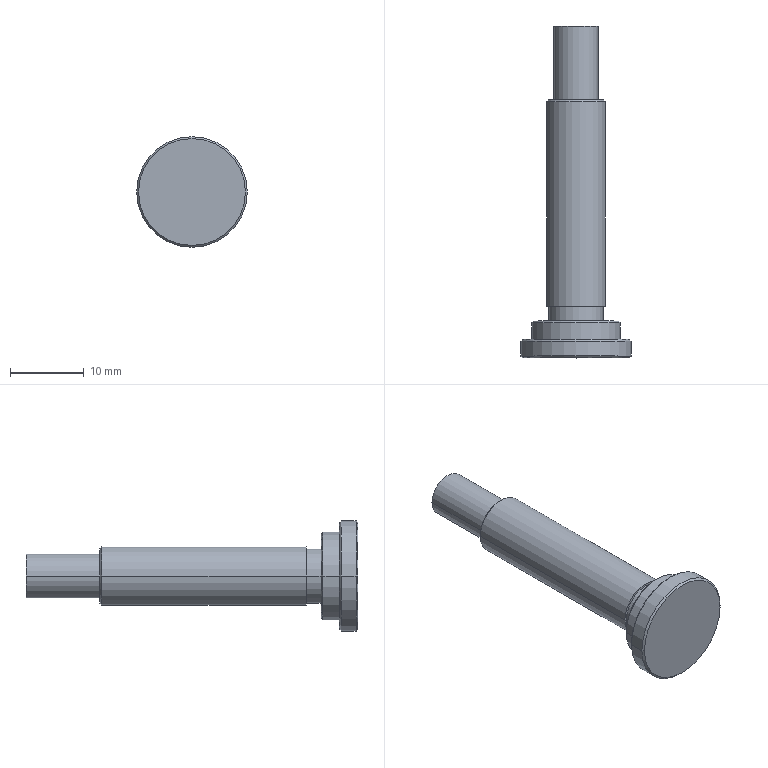Part | STEP file | Small pulley shaft | 1 solid | 24 faces | box 15 x 45 x 15 mm | volume 2496 mm3 | cylinder 10 | cone 8 | plane 6 | commonest cylinder face diameters 6 x2 7.4 x2 8 x2 12 x2 15 x2
STEP:
#1=CARTESIAN_POINT('',(0.,0.,0.));
#2=DIRECTION('',(0.,0.,1.));
#3=DIRECTION('',(1.,0.,0.));
#4=AXIS2_PLACEMENT_3D('',#1,#2,#3);
#5=CARTESIAN_POINT('',(-3.75,35.,0.));
#6=VERTEX_POINT('',#5);
#7=CARTESIAN_POINT('',(3.75,35.,0.));
#8=VERTEX_POINT('',#7);
#9=CARTESIAN_POINT('',(0.,35.,0.));
#10=DIRECTION('',(0.,1.,0.));
#11=DIRECTION('',(1.,0.,0.));
#12=AXIS2_PLACEMENT_3D('',#9,#10,#11);
#13=CIRCLE('',#12,3.75);
#14=CARTESIAN_POINT('',(0.,34.75,0.));
#15=DIRECTION('',(0.,-1.,0.));
#16=DIRECTION('',(1.,0.,0.));
#17=AXIS2_PLACEMENT_3D('',#14,#15,#16);
#18=CONICAL_SURFACE('',#17,4.,0.7854);
#19=CARTESIAN_POINT('',(6.283,-0.25));
#20=DIRECTION('',(-1.,0.));
#21=VECTOR('',#20,1.);
#22=LINE('',#19,#21);
#23=(GEOMETRIC_REPRESENTATION_CONTEXT(2)PARAMETRIC_REPRESENTATION_CONTEXT()REPRESENTATION_CONTEXT('',''));
#24=DEFINITIONAL_REPRESENTATION('',(#22),#23);
#25=PCURVE('',#18,#24);
#26=CARTESIAN_POINT('',(-3.,35.,0.));
#27=DIRECTION('',(0.,-1.,0.));
#28=DIRECTION('',(1.,0.,0.));
#29=AXIS2_PLACEMENT_3D('',#26,#27,#28);
#30=PLANE('',#29);
#31=CARTESIAN_POINT('',(6.75,0.));
#32=CARTESIAN_POINT('',(6.75,-6.495));
#33=CARTESIAN_POINT('',(1.125,-3.248));
#34=CARTESIAN_POINT('',(-4.5,0.));
#35=CARTESIAN_POINT('',(1.125,3.248));
#36=CARTESIAN_POINT('',(6.75,6.495));
#37=CARTESIAN_POINT('',(6.75,0.));
#38=(BOUNDED_CURVE()B_SPLINE_CURVE(2,(#31,#32,#33,#34,#35,#36,#37),.UNSPECIFIED.,.T.,.F.)B_SPLINE_CURVE_WITH_KNOTS((1,2,2,2,2,1),(-2.094,0.,2.094,4.189,6.283,8.378),.UNSPECIFIED.)CURVE()GEOMETRIC_REPRESENTATION_ITEM()RATIONAL_B_SPLINE_CURVE((1.,0.5,1.,0.5,1.,0.5,1.))REPRESENTATION_ITEM(''));
#39=(GEOMETRIC_REPRESENTATION_CONTEXT(2)PARAMETRIC_REPRESENTATION_CONTEXT()REPRESENTATION_CONTEXT('',''));
#40=DEFINITIONAL_REPRESENTATION('',(#38),#39);
#41=PCURVE('',#30,#40);
#42=SURFACE_CURVE('',#13,(#25,#41),.PCURVE_S1.);
#43=EDGE_CURVE('',#6,#8,#42,.T.);
#44=ORIENTED_EDGE('',*,*,#43,.F.);
#45=CARTESIAN_POINT('',(-4.,34.75,0.));
#46=VERTEX_POINT('',#45);
#47=CARTESIAN_POINT('',(-4.,34.75,0.));
#48=DIRECTION('',(-0.7071,-0.7071,0.));
#49=VECTOR('',#48,1.);
#50=LINE('',#47,#49);
#51=CARTESIAN_POINT('',(3.142,0.));
#52=DIRECTION('',(0.,1.));
#53=VECTOR('',#52,1.);
#54=LINE('',#51,#53);
#55=(GEOMETRIC_REPRESENTATION_CONTEXT(2)PARAMETRIC_REPRESENTATION_CONTEXT()REPRESENTATION_CONTEXT('',''));
#56=DEFINITIONAL_REPRESENTATION('',(#54),#55);
#57=PCURVE('',#18,#56);
#58=CARTESIAN_POINT('',(0.,34.75,0.));
#59=DIRECTION('',(0.,-1.,0.));
#60=DIRECTION('',(1.,0.,0.));
#61=AXIS2_PLACEMENT_3D('',#58,#59,#60);
#62=CONICAL_SURFACE('',#61,4.,0.7854);
#63=CARTESIAN_POINT('',(3.142,0.));
#64=DIRECTION('',(0.,1.));
#65=VECTOR('',#64,1.);
#66=LINE('',#63,#65);
#67=(GEOMETRIC_REPRESENTATION_CONTEXT(2)PARAMETRIC_REPRESENTATION_CONTEXT()REPRESENTATION_CONTEXT('',''));
#68=DEFINITIONAL_REPRESENTATION('',(#66),#67);
#69=PCURVE('',#62,#68);
#70=SURFACE_CURVE('',#50,(#57,#69),.PCURVE_S1.);
#71=EDGE_CURVE('',#6,#46,#70,.T.);
#72=ORIENTED_EDGE('',*,*,#71,.T.);
#73=CARTESIAN_POINT('',(4.,34.75,0.));
#74=VERTEX_POINT('',#73);
#75=CARTESIAN_POINT('',(0.,34.75,0.));
#76=DIRECTION('',(0.,-1.,0.));
#77=DIRECTION('',(1.,0.,0.));
#78=AXIS2_PLACEMENT_3D('',#75,#76,#77);
#79=CIRCLE('',#78,4.);
#80=CARTESIAN_POINT('',(0.,0.));
#81=DIRECTION('',(1.,0.));
#82=VECTOR('',#81,1.);
#83=LINE('',#80,#82);
#84=(GEOMETRIC_REPRESENTATION_CONTEXT(2)PARAMETRIC_REPRESENTATION_CONTEXT()REPRESENTATION_CONTEXT('',''));
#85=DEFINITIONAL_REPRESENTATION('',(#83),#84);
#86=PCURVE('',#18,#85);
#87=CARTESIAN_POINT('',(0.,0.,0.));
#88=DIRECTION('',(0.,-1.,0.));
#89=DIRECTION('',(1.,0.,0.));
#90=AXIS2_PLACEMENT_3D('',#87,#88,#89);
#91=CYLINDRICAL_SURFACE('',#90,4.);
#92=CARTESIAN_POINT('',(0.,-34.75));
#93=DIRECTION('',(1.,0.));
#94=VECTOR('',#93,1.);
#95=LINE('',#92,#94);
#96=(GEOMETRIC_REPRESENTATION_CONTEXT(2)PARAMETRIC_REPRESENTATION_CONTEXT()REPRESENTATION_CONTEXT('',''));
#97=DEFINITIONAL_REPRESENTATION('',(#95),#96);
#98=PCURVE('',#91,#97);
#99=SURFACE_CURVE('',#79,(#86,#98),.PCURVE_S1.);
#100=EDGE_CURVE('',#74,#46,#99,.T.);
#101=ORIENTED_EDGE('',*,*,#100,.F.);
#102=CARTESIAN_POINT('',(4.,34.75,0.));
#103=DIRECTION('',(0.7071,-0.7071,0.));
#104=VECTOR('',#103,1.);
#105=LINE('',#102,#104);
#106=CARTESIAN_POINT('',(0.,0.));
#107=DIRECTION('',(0.,1.));
#108=VECTOR('',#107,1.);
#109=LINE('',#106,#108);
#110=(GEOMETRIC_REPRESENTATION_CONTEXT(2)PARAMETRIC_REPRESENTATION_CONTEXT()REPRESENTATION_CONTEXT('',''));
#111=DEFINITIONAL_REPRESENTATION('',(#109),#110);
#112=PCURVE('',#18,#111);
#113=CARTESIAN_POINT('',(6.283,0.));
#114=DIRECTION('',(0.,1.));
#115=VECTOR('',#114,1.);
#116=LINE('',#113,#115);
#117=(GEOMETRIC_REPRESENTATION_CONTEXT(2)PARAMETRIC_REPRESENTATION_CONTEXT()REPRESENTATION_CONTEXT('',''));
#118=DEFINITIONAL_REPRESENTATION('',(#116),#117);
#119=PCURVE('',#62,#118);
#120=SURFACE_CURVE('',#105,(#112,#119),.PCURVE_S1.);
#121=EDGE_CURVE('',#8,#74,#120,.T.);
#122=ORIENTED_EDGE('',*,*,#121,.F.);
#123=EDGE_LOOP('',(#44,#72,#101,#122));
#124=FACE_BOUND('',#123,.T.);
#125=ADVANCED_FACE('',(#124),#18,.T.);
#126=CARTESIAN_POINT('',(-7.25,2.5,0.));
#127=VERTEX_POINT('',#126);
#128=CARTESIAN_POINT('',(7.25,2.5,0.));
#129=VERTEX_POINT('',#128);
#130=CARTESIAN_POINT('',(0.,2.5,0.));
#131=DIRECTION('',(0.,1.,0.));
#132=DIRECTION('',(1.,0.,0.));
#133=AXIS2_PLACEMENT_3D('',#130,#131,#132);
#134=CIRCLE('',#133,7.25);
#135=CARTESIAN_POINT('',(0.,2.25,0.));
#136=DIRECTION('',(0.,-1.,0.));
#137=DIRECTION('',(1.,0.,0.));
#138=AXIS2_PLACEMENT_3D('',#135,#136,#137);
#139=CONICAL_SURFACE('',#138,7.5,0.7854);
#140=CARTESIAN_POINT('',(6.283,-0.25));
#141=DIRECTION('',(-1.,0.));
#142=VECTOR('',#141,1.);
#143=LINE('',#140,#142);
#144=(GEOMETRIC_REPRESENTATION_CONTEXT(2)PARAMETRIC_REPRESENTATION_CONTEXT()REPRESENTATION_CONTEXT('',''));
#145=DEFINITIONAL_REPRESENTATION('',(#143),#144);
#146=PCURVE('',#139,#145);
#147=CARTESIAN_POINT('',(-6.,2.5,0.));
#148=DIRECTION('',(0.,-1.,0.));
#149=DIRECTION('',(1.,0.,0.));
#150=AXIS2_PLACEMENT_3D('',#147,#148,#149);
#151=PLANE('',#150);
#152=CARTESIAN_POINT('',(13.25,0.));
#153=CARTESIAN_POINT('',(13.25,-12.557));
#154=CARTESIAN_POINT('',(2.375,-6.279));
#155=CARTESIAN_POINT('',(-8.5,0.));
#156=CARTESIAN_POINT('',(2.375,6.279));
#157=CARTESIAN_POINT('',(13.25,12.557));
#158=CARTESIAN_POINT('',(13.25,0.));
#159=(BOUNDED_CURVE()B_SPLINE_CURVE(2,(#152,#153,#154,#155,#156,#157,#158),.UNSPECIFIED.,.T.,.F.)B_SPLINE_CURVE_WITH_KNOTS((1,2,2,2,2,1),(-2.094,0.,2.094,4.189,6.283,8.378),.UNSPECIFIED.)CURVE()GEOMETRIC_REPRESENTATION_ITEM()RATIONAL_B_SPLINE_CURVE((1.,0.5,1.,0.5,1.,0.5,1.))REPRESENTATION_ITEM(''));
#160=(GEOMETRIC_REPRESENTATION_CONTEXT(2)PARAMETRIC_REPRESENTATION_CONTEXT()REPRESENTATION_CONTEXT('',''));
#161=DEFINITIONAL_REPRESENTATION('',(#159),#160);
#162=PCURVE('',#151,#161);
#163=SURFACE_CURVE('',#134,(#146,#162),.PCURVE_S1.);
#164=EDGE_CURVE('',#127,#129,#163,.T.);
#165=ORIENTED_EDGE('',*,*,#164,.F.);
#166=CARTESIAN_POINT('',(-7.5,2.25,0.));
#167=VERTEX_POINT('',#166);
#168=CARTESIAN_POINT('',(-7.5,2.25,0.));
#169=DIRECTION('',(-0.7071,-0.7071,0.));
#170=VECTOR('',#169,1.);
#171=LINE('',#168,#170);
#172=CARTESIAN_POINT('',(3.142,0.));
#173=DIRECTION('',(0.,1.));
#174=VECTOR('',#173,1.);
#175=LINE('',#172,#174);
#176=(GEOMETRIC_REPRESENTATION_CONTEXT(2)PARAMETRIC_REPRESENTATION_CONTEXT()REPRESENTATION_CONTEXT('',''));
#177=DEFINITIONAL_REPRESENTATION('',(#175),#176);
#178=PCURVE('',#139,#177);
#179=CARTESIAN_POINT('',(0.,2.25,0.));
#180=DIRECTION('',(0.,-1.,0.));
#181=DIRECTION('',(1.,0.,0.));
#182=AXIS2_PLACEMENT_3D('',#179,#180,#181);
#183=CONICAL_SURFACE('',#182,7.5,0.7854);
#184=CARTESIAN_POINT('',(3.142,0.));
#185=DIRECTION('',(0.,1.));
#186=VECTOR('',#185,1.);
#187=LINE('',#184,#186);
#188=(GEOMETRIC_REPRESENTATION_CONTEXT(2)PARAMETRIC_REPRESENTATION_CONTEXT()REPRESENTATION_CONTEXT('',''));
#189=DEFINITIONAL_REPRESENTATION('',(#187),#188);
#190=PCURVE('',#183,#189);
#191=SURFACE_CURVE('',#171,(#178,#190),.PCURVE_S1.);
#192=EDGE_CURVE('',#127,#167,#191,.T.);
#193=ORIENTED_EDGE('',*,*,#192,.T.);
#194=CARTESIAN_POINT('',(7.5,2.25,0.));
#195=VERTEX_POINT('',#194);
#196=CARTESIAN_POINT('',(0.,2.25,0.));
#197=DIRECTION('',(0.,-1.,0.));
#198=DIRECTION('',(1.,0.,0.));
#199=AXIS2_PLACEMENT_3D('',#196,#197,#198);
#200=CIRCLE('',#199,7.5);
#201=CARTESIAN_POINT('',(0.,0.));
#202=DIRECTION('',(1.,0.));
#203=VECTOR('',#202,1.);
#204=LINE('',#201,#203);
#205=(GEOMETRIC_REPRESENTATION_CONTEXT(2)PARAMETRIC_REPRESENTATION_CONTEXT()REPRESENTATION_CONTEXT('',''));
#206=DEFINITIONAL_REPRESENTATION('',(#204),#205);
#207=PCURVE('',#139,#206);
#208=CARTESIAN_POINT('',(0.,0.,0.));
#209=DIRECTION('',(0.,-1.,0.));
#210=DIRECTION('',(1.,0.,0.));
#211=AXIS2_PLACEMENT_3D('',#208,#209,#210);
#212=CYLINDRICAL_SURFACE('',#211,7.5);
#213=CARTESIAN_POINT('',(0.,-2.25));
#214=DIRECTION('',(1.,0.));
#215=VECTOR('',#214,1.);
#216=LINE('',#213,#215);
#217=(GEOMETRIC_REPRESENTATION_CONTEXT(2)PARAMETRIC_REPRESENTATION_CONTEXT()REPRESENTATION_CONTEXT('',''));
#218=DEFINITIONAL_REPRESENTATION('',(#216),#217);
#219=PCURVE('',#212,#218);
#220=SURFACE_CURVE('',#200,(#207,#219),.PCURVE_S1.);
#221=EDGE_CURVE('',#195,#167,#220,.T.);
#222=ORIENTED_EDGE('',*,*,#221,.F.);
#223=CARTESIAN_POINT('',(7.5,2.25,0.));
#224=DIRECTION('',(0.7071,-0.7071,0.));
#225=VECTOR('',#224,1.);
#226=LINE('',#223,#225);
#227=CARTESIAN_POINT('',(0.,0.));
#228=DIRECTION('',(0.,1.));
#229=VECTOR('',#228,1.);
#230=LINE('',#227,#229);
#231=(GEOMETRIC_REPRESENTATION_CONTEXT(2)PARAMETRIC_REPRESENTATION_CONTEXT()REPRESENTATION_CONTEXT('',''));
#232=DEFINITIONAL_REPRESENTATION('',(#230),#231);
#233=PCURVE('',#139,#232);
#234=CARTESIAN_POINT('',(6.283,0.));
#235=DIRECTION('',(0.,1.));
#236=VECTOR('',#235,1.);
#237=LINE('',#234,#236);
#238=(GEOMETRIC_REPRESENTATION_CONTEXT(2)PARAMETRIC_REPRESENTATION_CONTEXT()REPRESENTATION_CONTEXT('',''));
#239=DEFINITIONAL_REPRESENTATION('',(#237),#238);
#240=PCURVE('',#183,#239);
#241=SURFACE_CURVE('',#226,(#233,#240),.PCURVE_S1.);
#242=EDGE_CURVE('',#129,#195,#241,.T.);
#243=ORIENTED_EDGE('',*,*,#242,.F.);
#244=EDGE_LOOP('',(#165,#193,#222,#243));
#245=FACE_BOUND('',#244,.T.);
#246=ADVANCED_FACE('',(#245),#139,.T.);
#247=CARTESIAN_POINT('',(7.25,0.,0.));
#248=VERTEX_POINT('',#247);
#249=CARTESIAN_POINT('',(-7.25,0.,0.));
#250=VERTEX_POINT('',#249);
#251=CARTESIAN_POINT('',(0.,0.,0.));
#252=DIRECTION('',(0.,-1.,0.));
#253=DIRECTION('',(-1.,0.,0.));
#254=AXIS2_PLACEMENT_3D('',#251,#252,#253);
#255=CIRCLE('',#254,7.25);
#256=CARTESIAN_POINT('',(0.,0.,0.));
#257=DIRECTION('',(0.,1.,0.));
#258=DIRECTION('',(-1.,0.,0.));
#259=AXIS2_PLACEMENT_3D('',#256,#257,#258);
#260=CONICAL_SURFACE('',#259,7.25,0.7854);
#261=CARTESIAN_POINT('',(6.283,0.));
#262=DIRECTION('',(-1.,0.));
#263=VECTOR('',#262,1.);
#264=LINE('',#261,#263);
#265=(GEOMETRIC_REPRESENTATION_CONTEXT(2)PARAMETRIC_REPRESENTATION_CONTEXT()REPRESENTATION_CONTEXT('',''));
#266=DEFINITIONAL_REPRESENTATION('',(#264),#265);
#267=PCURVE('',#260,#266);
#268=CARTESIAN_POINT('',(-7.5,0.,0.));
#269=DIRECTION('',(0.,1.,0.));
#270=DIRECTION('',(-1.,0.,0.));
#271=AXIS2_PLACEMENT_3D('',#268,#269,#270);
#272=PLANE('',#271);
#273=CARTESIAN_POINT('',(-0.25,0.));
#274=CARTESIAN_POINT('',(-0.25,-12.557));
#275=CARTESIAN_POINT('',(-11.125,-6.279));
#276=CARTESIAN_POINT('',(-22.,0.));
#277=CARTESIAN_POINT('',(-11.125,6.279));
#278=CARTESIAN_POINT('',(-0.25,12.557));
#279=CARTESIAN_POINT('',(-0.25,0.));
#280=(BOUNDED_CURVE()B_SPLINE_CURVE(2,(#273,#274,#275,#276,#277,#278,#279),.UNSPECIFIED.,.T.,.F.)B_SPLINE_CURVE_WITH_KNOTS((1,2,2,2,2,1),(-2.094,0.,2.094,4.189,6.283,8.378),.UNSPECIFIED.)CURVE()GEOMETRIC_REPRESENTATION_ITEM()RATIONAL_B_SPLINE_CURVE((1.,0.5,1.,0.5,1.,0.5,1.))REPRESENTATION_ITEM(''));
#281=(GEOMETRIC_REPRESENTATION_CONTEXT(2)PARAMETRIC_REPRESENTATION_CONTEXT()REPRESENTATION_CONTEXT('',''));
#282=DEFINITIONAL_REPRESENTATION('',(#280),#281);
#283=PCURVE('',#272,#282);
#284=SURFACE_CURVE('',#255,(#267,#283),.PCURVE_S1.);
#285=EDGE_CURVE('',#248,#250,#284,.T.);
#286=ORIENTED_EDGE('',*,*,#285,.F.);
#287=CARTESIAN_POINT('',(7.5,0.25,0.));
#288=VERTEX_POINT('',#287);
#289=CARTESIAN_POINT('',(7.25,0.,0.));
#290=DIRECTION('',(0.7071,0.7071,0.));
#291=VECTOR('',#290,1.);
#292=LINE('',#289,#291);
#293=CARTESIAN_POINT('',(3.142,0.));
#294=DIRECTION('',(0.,1.));
#295=VECTOR('',#294,1.);
#296=LINE('',#293,#295);
#297=(GEOMETRIC_REPRESENTATION_CONTEXT(2)PARAMETRIC_REPRESENTATION_CONTEXT()REPRESENTATION_CONTEXT('',''));
#298=DEFINITIONAL_REPRESENTATION('',(#296),#297);
#299=PCURVE('',#260,#298);
#300=CARTESIAN_POINT('',(0.,0.,0.));
#301=DIRECTION('',(0.,1.,0.));
#302=DIRECTION('',(-1.,0.,0.));
#303=AXIS2_PLACEMENT_3D('',#300,#301,#302);
#304=CONICAL_SURFACE('',#303,7.25,0.7854);
#305=CARTESIAN_POINT('',(3.142,0.));
#306=DIRECTION('',(0.,1.));
#307=VECTOR('',#306,1.);
#308=LINE('',#305,#307);
#309=(GEOMETRIC_REPRESENTATION_CONTEXT(2)PARAMETRIC_REPRESENTATION_CONTEXT()REPRESENTATION_CONTEXT('',''));
#310=DEFINITIONAL_REPRESENTATION('',(#308),#309);
#311=PCURVE('',#304,#310);
#312=SURFACE_CURVE('',#292,(#299,#311),.PCURVE_S1.);
#313=EDGE_CURVE('',#248,#288,#312,.T.);
#314=ORIENTED_EDGE('',*,*,#313,.T.);
#315=CARTESIAN_POINT('',(-7.5,0.25,0.));
#316=VERTEX_POINT('',#315);
#317=CARTESIAN_POINT('',(0.,0.25,0.));
#318=DIRECTION('',(0.,1.,0.));
#319=DIRECTION('',(-1.,0.,0.));
#320=AXIS2_PLACEMENT_3D('',#317,#318,#319);
#321=CIRCLE('',#320,7.5);
#322=CARTESIAN_POINT('',(0.,0.25));
#323=DIRECTION('',(1.,0.));
#324=VECTOR('',#323,1.);
#325=LINE('',#322,#324);
#326=(GEOMETRIC_REPRESENTATION_CONTEXT(2)PARAMETRIC_REPRESENTATION_CONTEXT()REPRESENTATION_CONTEXT('',''));
#327=DEFINITIONAL_REPRESENTATION('',(#325),#326);
#328=PCURVE('',#260,#327);
#329=CARTESIAN_POINT('',(3.142,-0.25));
#330=DIRECTION('',(-1.,0.));
#331=VECTOR('',#330,1.);
#332=LINE('',#329,#331);
#333=(GEOMETRIC_REPRESENTATION_CONTEXT(2)PARAMETRIC_REPRESENTATION_CONTEXT()REPRESENTATION_CONTEXT('',''));
#334=DEFINITIONAL_REPRESENTATION('',(#332),#333);
#335=PCURVE('',#212,#334);
#336=SURFACE_CURVE('',#321,(#328,#335),.PCURVE_S1.);
#337=EDGE_CURVE('',#316,#288,#336,.T.);
#338=ORIENTED_EDGE('',*,*,#337,.F.);
#339=CARTESIAN_POINT('',(-7.25,0.,0.));
#340=DIRECTION('',(-0.7071,0.7071,0.));
#341=VECTOR('',#340,1.);
#342=LINE('',#339,#341);
#343=CARTESIAN_POINT('',(0.,0.));
#344=DIRECTION('',(0.,1.));
#345=VECTOR('',#344,1.);
#346=LINE('',#343,#345);
#347=(GEOMETRIC_REPRESENTATION_CONTEXT(2)PARAMETRIC_REPRESENTATION_CONTEXT()REPRESENTATION_CONTEXT('',''));
#348=DEFINITIONAL_REPRESENTATION('',(#346),#347);
#349=PCURVE('',#260,#348);
#350=CARTESIAN_POINT('',(6.283,0.));
#351=DIRECTION('',(0.,1.));
#352=VECTOR('',#351,1.);
#353=LINE('',#350,#352);
#354=(GEOMETRIC_REPRESENTATION_CONTEXT(2)PARAMETRIC_REPRESENTATION_CONTEXT()REPRESENTATION_CONTEXT('',''));
#355=DEFINITIONAL_REPRESENTATION('',(#353),#354);
#356=PCURVE('',#304,#355);
#357=SURFACE_CURVE('',#342,(#349,#356),.PCURVE_S1.);
#358=EDGE_CURVE('',#250,#316,#357,.T.);
#359=ORIENTED_EDGE('',*,*,#358,.F.);
#360=EDGE_LOOP('',(#286,#314,#338,#359));
#361=FACE_BOUND('',#360,.T.);
#362=ADVANCED_FACE('',(#361),#260,.T.);
#363=CARTESIAN_POINT('',(-5.75,5.,0.));
#364=VERTEX_POINT('',#363);
#365=CARTESIAN_POINT('',(5.75,5.,0.));
#366=VERTEX_POINT('',#365);
#367=CARTESIAN_POINT('',(0.,5.,0.));
#368=DIRECTION('',(0.,1.,0.));
#369=DIRECTION('',(1.,0.,0.));
#370=AXIS2_PLACEMENT_3D('',#367,#368,#369);
#371=CIRCLE('',#370,5.75);
#372=CARTESIAN_POINT('',(0.,4.75,0.));
#373=DIRECTION('',(0.,-1.,0.));
#374=DIRECTION('',(1.,0.,0.));
#375=AXIS2_PLACEMENT_3D('',#372,#373,#374);
#376=CONICAL_SURFACE('',#375,6.,0.7854);
#377=CARTESIAN_POINT('',(6.283,-0.25));
#378=DIRECTION('',(-1.,0.));
#379=VECTOR('',#378,1.);
#380=LINE('',#377,#379);
#381=(GEOMETRIC_REPRESENTATION_CONTEXT(2)PARAMETRIC_REPRESENTATION_CONTEXT()REPRESENTATION_CONTEXT('',''));
#382=DEFINITIONAL_REPRESENTATION('',(#380),#381);
#383=PCURVE('',#376,#382);
#384=CARTESIAN_POINT('',(-4.,5.,0.));
#385=DIRECTION('',(0.,-1.,0.));
#386=DIRECTION('',(1.,0.,0.));
#387=AXIS2_PLACEMENT_3D('',#384,#385,#386);
#388=PLANE('',#387);
#389=CARTESIAN_POINT('',(9.75,0.));
#390=CARTESIAN_POINT('',(9.75,-9.959));
#391=CARTESIAN_POINT('',(1.125,-4.98));
#392=CARTESIAN_POINT('',(-7.5,0.));
#393=CARTESIAN_POINT('',(1.125,4.98));
#394=CARTESIAN_POINT('',(9.75,9.959));
#395=CARTESIAN_POINT('',(9.75,0.));
#396=(BOUNDED_CURVE()B_SPLINE_CURVE(2,(#389,#390,#391,#392,#393,#394,#395),.UNSPECIFIED.,.T.,.F.)B_SPLINE_CURVE_WITH_KNOTS((1,2,2,2,2,1),(-2.094,0.,2.094,4.189,6.283,8.378),.UNSPECIFIED.)CURVE()GEOMETRIC_REPRESENTATION_ITEM()RATIONAL_B_SPLINE_CURVE((1.,0.5,1.,0.5,1.,0.5,1.))REPRESENTATION_ITEM(''));
#397=(GEOMETRIC_REPRESENTATION_CONTEXT(2)PARAMETRIC_REPRESENTATION_CONTEXT()REPRESENTATION_CONTEXT('',''));
#398=DEFINITIONAL_REPRESENTATION('',(#396),#397);
#399=PCURVE('',#388,#398);
#400=SURFACE_CURVE('',#371,(#383,#399),.PCURVE_S1.);
#401=EDGE_CURVE('',#364,#366,#400,.T.);
#402=ORIENTED_EDGE('',*,*,#401,.F.);
#403=CARTESIAN_POINT('',(-6.,4.75,0.));
#404=VERTEX_POINT('',#403);
#405=CARTESIAN_POINT('',(-6.,4.75,0.));
#406=DIRECTION('',(-0.7071,-0.7071,0.));
#407=VECTOR('',#406,1.);
#408=LINE('',#405,#407);
#409=CARTESIAN_POINT('',(3.142,0.));
#410=DIRECTION('',(0.,1.));
#411=VECTOR('',#410,1.);
#412=LINE('',#409,#411);
#413=(GEOMETRIC_REPRESENTATION_CONTEXT(2)PARAMETRIC_REPRESENTATION_CONTEXT()REPRESENTATION_CONTEXT('',''));
#414=DEFINITIONAL_REPRESENTATION('',(#412),#413);
#415=PCURVE('',#376,#414);
#416=CARTESIAN_POINT('',(0.,4.75,0.));
#417=DIRECTION('',(0.,-1.,0.));
#418=DIRECTION('',(1.,0.,0.));
#419=AXIS2_PLACEMENT_3D('',#416,#417,#418);
#420=CONICAL_SURFACE('',#419,6.,0.7854);
#421=CARTESIAN_POINT('',(3.142,0.));
#422=DIRECTION('',(0.,1.));
#423=VECTOR('',#422,1.);
#424=LINE('',#421,#423);
#425=(GEOMETRIC_REPRESENTATION_CONTEXT(2)PARAMETRIC_REPRESENTATION_CONTEXT()REPRESENTATION_CONTEXT('',''));
#426=DEFINITIONAL_REPRESENTATION('',(#424),#425);
#427=PCURVE('',#420,#426);
#428=SURFACE_CURVE('',#408,(#415,#427),.PCURVE_S1.);
#429=EDGE_CURVE('',#364,#404,#428,.T.);
#430=ORIENTED_EDGE('',*,*,#429,.T.);
#431=CARTESIAN_POINT('',(6.,4.75,0.));
#432=VERTEX_POINT('',#431);
#433=CARTESIAN_POINT('',(0.,4.75,0.));
#434=DIRECTION('',(0.,-1.,0.));
#435=DIRECTION('',(1.,0.,0.));
#436=AXIS2_PLACEMENT_3D('',#433,#434,#435);
#437=CIRCLE('',#436,6.);
#438=CARTESIAN_POINT('',(0.,0.));
#439=DIRECTION('',(1.,0.));
#440=VECTOR('',#439,1.);
#441=LINE('',#438,#440);
#442=(GEOMETRIC_REPRESENTATION_CONTEXT(2)PARAMETRIC_REPRESENTATION_CONTEXT()REPRESENTATION_CONTEXT('',''));
#443=DEFINITIONAL_REPRESENTATION('',(#441),#442);
#444=PCURVE('',#376,#443);
#445=CARTESIAN_POINT('',(0.,0.,0.));
#446=DIRECTION('',(0.,-1.,0.));
#447=DIRECTION('',(1.,0.,0.));
#448=AXIS2_PLACEMENT_3D('',#445,#446,#447);
#449=CYLINDRICAL_SURFACE('',#448,6.);
#450=CARTESIAN_POINT('',(0.,-4.75));
#451=DIRECTION('',(1.,0.));
#452=VECTOR('',#451,1.);
#453=LINE('',#450,#452);
#454=(GEOMETRIC_REPRESENTATION_CONTEXT(2)PARAMETRIC_REPRESENTATION_CONTEXT()REPRESENTATION_CONTEXT('',''));
#455=DEFINITIONAL_REPRESENTATION('',(#453),#454);
#456=PCURVE('',#449,#455);
#457=SURFACE_CURVE('',#437,(#444,#456),.PCURVE_S1.);
#458=EDGE_CURVE('',#432,#404,#457,.T.);
#459=ORIENTED_EDGE('',*,*,#458,.F.);
#460=CARTESIAN_POINT('',(6.,4.75,0.));
#461=DIRECTION('',(0.7071,-0.7071,0.));
#462=VECTOR('',#461,1.);
#463=LINE('',#460,#462);
#464=CARTESIAN_POINT('',(0.,0.));
#465=DIRECTION('',(0.,1.));
#466=VECTOR('',#465,1.);
#467=LINE('',#464,#466);
#468=(GEOMETRIC_REPRESENTATION_CONTEXT(2)PARAMETRIC_REPRESENTATION_CONTEXT()REPRESENTATION_CONTEXT('',''));
#469=DEFINITIONAL_REPRESENTATION('',(#467),#468);
#470=PCURVE('',#376,#469);
#471=CARTESIAN_POINT('',(6.283,0.));
#472=DIRECTION('',(0.,1.));
#473=VECTOR('',#472,1.);
#474=LINE('',#471,#473);
#475=(GEOMETRIC_REPRESENTATION_CONTEXT(2)PARAMETRIC_REPRESENTATION_CONTEXT()REPRESENTATION_CONTEXT('',''));
#476=DEFINITIONAL_REPRESENTATION('',(#474),#475);
#477=PCURVE('',#420,#476);
#478=SURFACE_CURVE('',#463,(#470,#477),.PCURVE_S1.);
#479=EDGE_CURVE('',#366,#432,#478,.T.);
#480=ORIENTED_EDGE('',*,*,#479,.F.);
#481=EDGE_LOOP('',(#402,#430,#459,#480));
#482=FACE_BOUND('',#481,.T.);
#483=ADVANCED_FACE('',(#482),#376,.T.);
#484=ORIENTED_EDGE('',*,*,#100,.T.);
#485=CARTESIAN_POINT('',(-4.,7.,0.));
#486=VERTEX_POINT('',#485);
#487=CARTESIAN_POINT('',(-4.,0.,0.));
#488=DIRECTION('',(0.,-1.,0.));
#489=VECTOR('',#488,1.);
#490=LINE('',#487,#489);
#491=CARTESIAN_POINT('',(3.142,0.));
#492=DIRECTION('',(0.,1.));
#493=VECTOR('',#492,1.);
#494=LINE('',#491,#493);
#495=(GEOMETRIC_REPRESENTATION_CONTEXT(2)PARAMETRIC_REPRESENTATION_CONTEXT()REPRESENTATION_CONTEXT('',''));
#496=DEFINITIONAL_REPRESENTATION('',(#494),#495);
#497=PCURVE('',#91,#496);
#498=CARTESIAN_POINT('',(0.,0.,0.));
#499=DIRECTION('',(0.,-1.,0.));
#500=DIRECTION('',(1.,0.,0.));
#501=AXIS2_PLACEMENT_3D('',#498,#499,#500);
#502=CYLINDRICAL_SURFACE('',#501,4.);
#503=CARTESIAN_POINT('',(3.142,0.));
#504=DIRECTION('',(0.,1.));
#505=VECTOR('',#504,1.);
#506=LINE('',#503,#505);
#507=(GEOMETRIC_REPRESENTATION_CONTEXT(2)PARAMETRIC_REPRESENTATION_CONTEXT()REPRESENTATION_CONTEXT('',''));
#508=DEFINITIONAL_REPRESENTATION('',(#506),#507);
#509=PCURVE('',#502,#508);
#510=SURFACE_CURVE('',#490,(#497,#509),.PCURVE_S1.);
#511=EDGE_CURVE('',#46,#486,#510,.T.);
#512=ORIENTED_EDGE('',*,*,#511,.T.);
#513=CARTESIAN_POINT('',(4.,7.,0.));
#514=VERTEX_POINT('',#513);
#515=CARTESIAN_POINT('',(0.,7.,0.));
#516=DIRECTION('',(0.,1.,0.));
#517=DIRECTION('',(-1.,0.,0.));
#518=AXIS2_PLACEMENT_3D('',#515,#516,#517);
#519=CIRCLE('',#518,4.);
#520=CARTESIAN_POINT('',(3.142,-7.));
#521=DIRECTION('',(-1.,0.));
#522=VECTOR('',#521,1.);
#523=LINE('',#520,#522);
#524=(GEOMETRIC_REPRESENTATION_CONTEXT(2)PARAMETRIC_REPRESENTATION_CONTEXT()REPRESENTATION_CONTEXT('',''));
#525=DEFINITIONAL_REPRESENTATION('',(#523),#524);
#526=PCURVE('',#91,#525);
#527=CARTESIAN_POINT('',(0.,7.,0.));
#528=DIRECTION('',(0.,1.,0.));
#529=DIRECTION('',(-1.,0.,0.));
#530=AXIS2_PLACEMENT_3D('',#527,#528,#529);
#531=PLANE('',#530);
#532=CARTESIAN_POINT('',(0.,0.));
#533=DIRECTION('',(1.,0.));
#534=AXIS2_PLACEMENT_2D('',#532,#533);
#535=CIRCLE('',#534,4.);
#536=(GEOMETRIC_REPRESENTATION_CONTEXT(2)PARAMETRIC_REPRESENTATION_CONTEXT()REPRESENTATION_CONTEXT('',''));
#537=DEFINITIONAL_REPRESENTATION('',(#535),#536);
#538=PCURVE('',#531,#537);
#539=SURFACE_CURVE('',#519,(#526,#538),.PCURVE_S1.);
#540=EDGE_CURVE('',#486,#514,#539,.T.);
#541=ORIENTED_EDGE('',*,*,#540,.T.);
#542=CARTESIAN_POINT('',(4.,0.,0.));
#543=DIRECTION('',(0.,-1.,0.));
#544=VECTOR('',#543,1.);
#545=LINE('',#542,#544);
#546=CARTESIAN_POINT('',(0.,0.));
#547=DIRECTION('',(0.,1.));
#548=VECTOR('',#547,1.);
#549=LINE('',#546,#548);
#550=(GEOMETRIC_REPRESENTATION_CONTEXT(2)PARAMETRIC_REPRESENTATION_CONTEXT()REPRESENTATION_CONTEXT('',''));
#551=DEFINITIONAL_REPRESENTATION('',(#549),#550);
#552=PCURVE('',#91,#551);
#553=CARTESIAN_POINT('',(6.283,0.));
#554=DIRECTION('',(0.,1.));
#555=VECTOR('',#554,1.);
#556=LINE('',#553,#555);
#557=(GEOMETRIC_REPRESENTATION_CONTEXT(2)PARAMETRIC_REPRESENTATION_CONTEXT()REPRESENTATION_CONTEXT('',''));
#558=DEFINITIONAL_REPRESENTATION('',(#556),#557);
#559=PCURVE('',#502,#558);
#560=SURFACE_CURVE('',#545,(#552,#559),.PCURVE_S1.);
#561=EDGE_CURVE('',#74,#514,#560,.T.);
#562=ORIENTED_EDGE('',*,*,#561,.F.);
#563=EDGE_LOOP('',(#484,#512,#541,#562));
#564=FACE_BOUND('',#563,.T.);
#565=ADVANCED_FACE('',(#564),#91,.T.);
#566=CARTESIAN_POINT('',(3.,45.,0.));
#567=VERTEX_POINT('',#566);
#568=CARTESIAN_POINT('',(-3.,45.,0.));
#569=VERTEX_POINT('',#568);
#570=CARTESIAN_POINT('',(0.,45.,0.));
#571=DIRECTION('',(0.,-1.,0.));
#572=DIRECTION('',(1.,0.,0.));
#573=AXIS2_PLACEMENT_3D('',#570,#571,#572);
#574=CIRCLE('',#573,3.);
#575=CARTESIAN_POINT('',(0.,0.,0.));
#576=DIRECTION('',(0.,-1.,0.));
#577=DIRECTION('',(1.,0.,0.));
#578=AXIS2_PLACEMENT_3D('',#575,#576,#577);
#579=CYLINDRICAL_SURFACE('',#578,3.);
#580=CARTESIAN_POINT('',(0.,-45.));
#581=DIRECTION('',(1.,0.));
#582=VECTOR('',#581,1.);
#583=LINE('',#580,#582);
#584=(GEOMETRIC_REPRESENTATION_CONTEXT(2)PARAMETRIC_REPRESENTATION_CONTEXT()REPRESENTATION_CONTEXT('',''));
#585=DEFINITIONAL_REPRESENTATION('',(#583),#584);
#586=PCURVE('',#579,#585);
#587=CARTESIAN_POINT('',(0.,45.,0.));
#588=DIRECTION('',(0.,-1.,0.));
#589=DIRECTION('',(1.,0.,0.));
#590=AXIS2_PLACEMENT_3D('',#587,#588,#589);
#591=PLANE('',#590);
#592=CARTESIAN_POINT('',(0.,0.));
#593=DIRECTION('',(1.,0.));
#594=AXIS2_PLACEMENT_2D('',#592,#593);
#595=CIRCLE('',#594,3.);
#596=(GEOMETRIC_REPRESENTATION_CONTEXT(2)PARAMETRIC_REPRESENTATION_CONTEXT()REPRESENTATION_CONTEXT('',''));
#597=DEFINITIONAL_REPRESENTATION('',(#595),#596);
#598=PCURVE('',#591,#597);
#599=SURFACE_CURVE('',#574,(#586,#598),.PCURVE_S1.);
#600=EDGE_CURVE('',#567,#569,#599,.T.);
#601=ORIENTED_EDGE('',*,*,#600,.T.);
#602=CARTESIAN_POINT('',(-3.,35.,0.));
#603=VERTEX_POINT('',#602);
#604=CARTESIAN_POINT('',(-3.,0.,0.));
#605=DIRECTION('',(0.,-1.,0.));
#606=VECTOR('',#605,1.);
#607=LINE('',#604,#606);
#608=CARTESIAN_POINT('',(3.142,0.));
#609=DIRECTION('',(0.,1.));
#610=VECTOR('',#609,1.);
#611=LINE('',#608,#610);
#612=(GEOMETRIC_REPRESENTATION_CONTEXT(2)PARAMETRIC_REPRESENTATION_CONTEXT()REPRESENTATION_CONTEXT('',''));
#613=DEFINITIONAL_REPRESENTATION('',(#611),#612);
#614=PCURVE('',#579,#613);
#615=CARTESIAN_POINT('',(0.,0.,0.));
#616=DIRECTION('',(0.,-1.,0.));
#617=DIRECTION('',(1.,0.,0.));
#618=AXIS2_PLACEMENT_3D('',#615,#616,#617);
#619=CYLINDRICAL_SURFACE('',#618,3.);
#620=CARTESIAN_POINT('',(3.142,0.));
#621=DIRECTION('',(0.,1.));
#622=VECTOR('',#621,1.);
#623=LINE('',#620,#622);
#624=(GEOMETRIC_REPRESENTATION_CONTEXT(2)PARAMETRIC_REPRESENTATION_CONTEXT()REPRESENTATION_CONTEXT('',''));
#625=DEFINITIONAL_REPRESENTATION('',(#623),#624);
#626=PCURVE('',#619,#625);
#627=SURFACE_CURVE('',#607,(#614,#626),.PCURVE_S1.);
#628=EDGE_CURVE('',#569,#603,#627,.T.);
#629=ORIENTED_EDGE('',*,*,#628,.T.);
#630=CARTESIAN_POINT('',(3.,35.,0.));
#631=VERTEX_POINT('',#630);
#632=CARTESIAN_POINT('',(0.,35.,0.));
#633=DIRECTION('',(0.,-1.,0.));
#634=DIRECTION('',(1.,0.,0.));
#635=AXIS2_PLACEMENT_3D('',#632,#633,#634);
#636=CIRCLE('',#635,3.);
#637=CARTESIAN_POINT('',(0.,-35.));
#638=DIRECTION('',(1.,0.));
#639=VECTOR('',#638,1.);
#640=LINE('',#637,#639);
#641=(GEOMETRIC_REPRESENTATION_CONTEXT(2)PARAMETRIC_REPRESENTATION_CONTEXT()REPRESENTATION_CONTEXT('',''));
#642=DEFINITIONAL_REPRESENTATION('',(#640),#641);
#643=PCURVE('',#579,#642);
#644=CARTESIAN_POINT('',(3.,0.));
#645=DIRECTION('',(1.,0.));
#646=AXIS2_PLACEMENT_2D('',#644,#645);
#647=CIRCLE('',#646,3.);
#648=(GEOMETRIC_REPRESENTATION_CONTEXT(2)PARAMETRIC_REPRESENTATION_CONTEXT()REPRESENTATION_CONTEXT('',''));
#649=DEFINITIONAL_REPRESENTATION('',(#647),#648);
#650=PCURVE('',#30,#649);
#651=SURFACE_CURVE('',#636,(#643,#650),.PCURVE_S1.);
#652=EDGE_CURVE('',#631,#603,#651,.T.);
#653=ORIENTED_EDGE('',*,*,#652,.F.);
#654=CARTESIAN_POINT('',(3.,0.,0.));
#655=DIRECTION('',(0.,-1.,0.));
#656=VECTOR('',#655,1.);
#657=LINE('',#654,#656);
#658=CARTESIAN_POINT('',(0.,0.));
#659=DIRECTION('',(0.,1.));
#660=VECTOR('',#659,1.);
#661=LINE('',#658,#660);
#662=(GEOMETRIC_REPRESENTATION_CONTEXT(2)PARAMETRIC_REPRESENTATION_CONTEXT()REPRESENTATION_CONTEXT('',''));
#663=DEFINITIONAL_REPRESENTATION('',(#661),#662);
#664=PCURVE('',#579,#663);
#665=CARTESIAN_POINT('',(6.283,0.));
#666=DIRECTION('',(0.,1.));
#667=VECTOR('',#666,1.);
#668=LINE('',#665,#667);
#669=(GEOMETRIC_REPRESENTATION_CONTEXT(2)PARAMETRIC_REPRESENTATION_CONTEXT()REPRESENTATION_CONTEXT('',''));
#670=DEFINITIONAL_REPRESENTATION('',(#668),#669);
#671=PCURVE('',#619,#670);
#672=SURFACE_CURVE('',#657,(#664,#671),.PCURVE_S1.);
#673=EDGE_CURVE('',#567,#631,#672,.T.);
#674=ORIENTED_EDGE('',*,*,#673,.F.);
#675=EDGE_LOOP('',(#601,#629,#653,#674));
#676=FACE_BOUND('',#675,.T.);
#677=ADVANCED_FACE('',(#676),#579,.T.);
#678=CARTESIAN_POINT('',(-3.7,7.,0.));
#679=VERTEX_POINT('',#678);
#680=CARTESIAN_POINT('',(3.7,7.,0.));
#681=VERTEX_POINT('',#680);
#682=CARTESIAN_POINT('',(0.,7.,0.));
#683=DIRECTION('',(0.,1.,0.));
#684=DIRECTION('',(-1.,0.,0.));
#685=AXIS2_PLACEMENT_3D('',#682,#683,#684);
#686=CIRCLE('',#685,3.7);
#687=CARTESIAN_POINT('',(0.,7.,0.));
#688=DIRECTION('',(0.,-1.,0.));
#689=DIRECTION('',(1.,0.,0.));
#690=AXIS2_PLACEMENT_3D('',#687,#688,#689);
#691=CYLINDRICAL_SURFACE('',#690,3.7);
#692=CARTESIAN_POINT('',(3.142,0.));
#693=DIRECTION('',(-1.,0.));
#694=VECTOR('',#693,1.);
#695=LINE('',#692,#694);
#696=(GEOMETRIC_REPRESENTATION_CONTEXT(2)PARAMETRIC_REPRESENTATION_CONTEXT()REPRESENTATION_CONTEXT('',''));
#697=DEFINITIONAL_REPRESENTATION('',(#695),#696);
#698=PCURVE('',#691,#697);
#699=CARTESIAN_POINT('',(0.,0.));
#700=DIRECTION('',(1.,0.));
#701=AXIS2_PLACEMENT_2D('',#699,#700);
#702=CIRCLE('',#701,3.7);
#703=(GEOMETRIC_REPRESENTATION_CONTEXT(2)PARAMETRIC_REPRESENTATION_CONTEXT()REPRESENTATION_CONTEXT('',''));
#704=DEFINITIONAL_REPRESENTATION('',(#702),#703);
#705=PCURVE('',#531,#704);
#706=SURFACE_CURVE('',#686,(#698,#705),.PCURVE_S1.);
#707=EDGE_CURVE('',#679,#681,#706,.T.);
#708=ORIENTED_EDGE('',*,*,#707,.F.);
#709=CARTESIAN_POINT('',(-3.7,5.,0.));
#710=VERTEX_POINT('',#709);
#711=CARTESIAN_POINT('',(-3.7,7.,0.));
#712=DIRECTION('',(0.,-1.,0.));
#713=VECTOR('',#712,1.);
#714=LINE('',#711,#713);
#715=CARTESIAN_POINT('',(3.142,0.));
#716=DIRECTION('',(0.,1.));
#717=VECTOR('',#716,1.);
#718=LINE('',#715,#717);
#719=(GEOMETRIC_REPRESENTATION_CONTEXT(2)PARAMETRIC_REPRESENTATION_CONTEXT()REPRESENTATION_CONTEXT('',''));
#720=DEFINITIONAL_REPRESENTATION('',(#718),#719);
#721=PCURVE('',#691,#720);
#722=CARTESIAN_POINT('',(0.,7.,0.));
#723=DIRECTION('',(0.,-1.,0.));
#724=DIRECTION('',(1.,0.,0.));
#725=AXIS2_PLACEMENT_3D('',#722,#723,#724);
#726=CYLINDRICAL_SURFACE('',#725,3.7);
#727=CARTESIAN_POINT('',(3.142,0.));
#728=DIRECTION('',(0.,1.));
#729=VECTOR('',#728,1.);
#730=LINE('',#727,#729);
#731=(GEOMETRIC_REPRESENTATION_CONTEXT(2)PARAMETRIC_REPRESENTATION_CONTEXT()REPRESENTATION_CONTEXT('',''));
#732=DEFINITIONAL_REPRESENTATION('',(#730),#731);
#733=PCURVE('',#726,#732);
#734=SURFACE_CURVE('',#714,(#721,#733),.PCURVE_S1.);
#735=EDGE_CURVE('',#679,#710,#734,.T.);
#736=ORIENTED_EDGE('',*,*,#735,.T.);
#737=CARTESIAN_POINT('',(3.7,5.,0.));
#738=VERTEX_POINT('',#737);
#739=CARTESIAN_POINT('',(0.,5.,0.));
#740=DIRECTION('',(0.,1.,0.));
#741=DIRECTION('',(-1.,0.,0.));
#742=AXIS2_PLACEMENT_3D('',#739,#740,#741);
#743=CIRCLE('',#742,3.7);
#744=CARTESIAN_POINT('',(3.142,2.));
#745=DIRECTION('',(-1.,0.));
#746=VECTOR('',#745,1.);
#747=LINE('',#744,#746);
#748=(GEOMETRIC_REPRESENTATION_CONTEXT(2)PARAMETRIC_REPRESENTATION_CONTEXT()REPRESENTATION_CONTEXT('',''));
#749=DEFINITIONAL_REPRESENTATION('',(#747),#748);
#750=PCURVE('',#691,#749);
#751=CARTESIAN_POINT('',(0.3,0.));
#752=CARTESIAN_POINT('',(0.3,6.409));
#753=CARTESIAN_POINT('',(5.85,3.204));
#754=CARTESIAN_POINT('',(11.4,0.));
#755=CARTESIAN_POINT('',(5.85,-3.204));
#756=CARTESIAN_POINT('',(0.3,-6.409));
#757=CARTESIAN_POINT('',(0.3,0.));
#758=(BOUNDED_CURVE()B_SPLINE_CURVE(2,(#751,#752,#753,#754,#755,#756,#757),.UNSPECIFIED.,.T.,.F.)B_SPLINE_CURVE_WITH_KNOTS((1,2,2,2,2,1),(-2.094,0.,2.094,4.189,6.283,8.378),.UNSPECIFIED.)CURVE()GEOMETRIC_REPRESENTATION_ITEM()RATIONAL_B_SPLINE_CURVE((1.,0.5,1.,0.5,1.,0.5,1.))REPRESENTATION_ITEM(''));
#759=(GEOMETRIC_REPRESENTATION_CONTEXT(2)PARAMETRIC_REPRESENTATION_CONTEXT()REPRESENTATION_CONTEXT('',''));
#760=DEFINITIONAL_REPRESENTATION('',(#758),#759);
#761=PCURVE('',#388,#760);
#762=SURFACE_CURVE('',#743,(#750,#761),.PCURVE_S1.);
#763=EDGE_CURVE('',#710,#738,#762,.T.);
#764=ORIENTED_EDGE('',*,*,#763,.T.);
#765=CARTESIAN_POINT('',(3.7,7.,0.));
#766=DIRECTION('',(0.,-1.,0.));
#767=VECTOR('',#766,1.);
#768=LINE('',#765,#767);
#769=CARTESIAN_POINT('',(0.,0.));
#770=DIRECTION('',(0.,1.));
#771=VECTOR('',#770,1.);
#772=LINE('',#769,#771);
#773=(GEOMETRIC_REPRESENTATION_CONTEXT(2)PARAMETRIC_REPRESENTATION_CONTEXT()REPRESENTATION_CONTEXT('',''));
#774=DEFINITIONAL_REPRESENTATION('',(#772),#773);
#775=PCURVE('',#691,#774);
#776=CARTESIAN_POINT('',(6.283,0.));
#777=DIRECTION('',(0.,1.));
#778=VECTOR('',#777,1.);
#779=LINE('',#776,#778);
#780=(GEOMETRIC_REPRESENTATION_CONTEXT(2)PARAMETRIC_REPRESENTATION_CONTEXT()REPRESENTATION_CONTEXT('',''));
#781=DEFINITIONAL_REPRESENTATION('',(#779),#780);
#782=PCURVE('',#726,#781);
#783=SURFACE_CURVE('',#768,(#775,#782),.PCURVE_S1.);
#784=EDGE_CURVE('',#681,#738,#783,.T.);
#785=ORIENTED_EDGE('',*,*,#784,.F.);
#786=EDGE_LOOP('',(#708,#736,#764,#785));
#787=FACE_BOUND('',#786,.T.);
#788=ADVANCED_FACE('',(#787),#691,.T.);
#789=ORIENTED_EDGE('',*,*,#221,.T.);
#790=CARTESIAN_POINT('',(-7.5,0.,0.));
#791=DIRECTION('',(0.,-1.,0.));
#792=VECTOR('',#791,1.);
#793=LINE('',#790,#792);
#794=CARTESIAN_POINT('',(3.142,0.));
#795=DIRECTION('',(0.,1.));
#796=VECTOR('',#795,1.);
#797=LINE('',#794,#796);
#798=(GEOMETRIC_REPRESENTATION_CONTEXT(2)PARAMETRIC_REPRESENTATION_CONTEXT()REPRESENTATION_CONTEXT('',''));
#799=DEFINITIONAL_REPRESENTATION('',(#797),#798);
#800=PCURVE('',#212,#799);
#801=CARTESIAN_POINT('',(0.,0.,0.));
#802=DIRECTION('',(0.,-1.,0.));
#803=DIRECTION('',(1.,0.,0.));
#804=AXIS2_PLACEMENT_3D('',#801,#802,#803);
#805=CYLINDRICAL_SURFACE('',#804,7.5);
#806=CARTESIAN_POINT('',(3.142,0.));
#807=DIRECTION('',(0.,1.));
#808=VECTOR('',#807,1.);
#809=LINE('',#806,#808);
#810=(GEOMETRIC_REPRESENTATION_CONTEXT(2)PARAMETRIC_REPRESENTATION_CONTEXT()REPRESENTATION_CONTEXT('',''));
#811=DEFINITIONAL_REPRESENTATION('',(#809),#810);
#812=PCURVE('',#805,#811);
#813=SURFACE_CURVE('',#793,(#800,#812),.PCURVE_S1.);
#814=EDGE_CURVE('',#167,#316,#813,.T.);
#815=ORIENTED_EDGE('',*,*,#814,.T.);
#816=ORIENTED_EDGE('',*,*,#337,.T.);
#817=CARTESIAN_POINT('',(7.5,0.,0.));
#818=DIRECTION('',(0.,-1.,0.));
#819=VECTOR('',#818,1.);
#820=LINE('',#817,#819);
#821=CARTESIAN_POINT('',(0.,0.));
#822=DIRECTION('',(0.,1.));
#823=VECTOR('',#822,1.);
#824=LINE('',#821,#823);
#825=(GEOMETRIC_REPRESENTATION_CONTEXT(2)PARAMETRIC_REPRESENTATION_CONTEXT()REPRESENTATION_CONTEXT('',''));
#826=DEFINITIONAL_REPRESENTATION('',(#824),#825);
#827=PCURVE('',#212,#826);
#828=CARTESIAN_POINT('',(6.283,0.));
#829=DIRECTION('',(0.,1.));
#830=VECTOR('',#829,1.);
#831=LINE('',#828,#830);
#832=(GEOMETRIC_REPRESENTATION_CONTEXT(2)PARAMETRIC_REPRESENTATION_CONTEXT()REPRESENTATION_CONTEXT('',''));
#833=DEFINITIONAL_REPRESENTATION('',(#831),#832);
#834=PCURVE('',#805,#833);
#835=SURFACE_CURVE('',#820,(#827,#834),.PCURVE_S1.);
#836=EDGE_CURVE('',#195,#288,#835,.T.);
#837=ORIENTED_EDGE('',*,*,#836,.F.);
#838=EDGE_LOOP('',(#789,#815,#816,#837));
#839=FACE_BOUND('',#838,.T.);
#840=ADVANCED_FACE('',(#839),#212,.T.);
#841=ORIENTED_EDGE('',*,*,#458,.T.);
#842=CARTESIAN_POINT('',(-6.,2.5,0.));
#843=VERTEX_POINT('',#842);
#844=CARTESIAN_POINT('',(-6.,0.,0.));
#845=DIRECTION('',(0.,-1.,0.));
#846=VECTOR('',#845,1.);
#847=LINE('',#844,#846);
#848=CARTESIAN_POINT('',(3.142,0.));
#849=DIRECTION('',(0.,1.));
#850=VECTOR('',#849,1.);
#851=LINE('',#848,#850);
#852=(GEOMETRIC_REPRESENTATION_CONTEXT(2)PARAMETRIC_REPRESENTATION_CONTEXT()REPRESENTATION_CONTEXT('',''));
#853=DEFINITIONAL_REPRESENTATION('',(#851),#852);
#854=PCURVE('',#449,#853);
#855=CARTESIAN_POINT('',(0.,0.,0.));
#856=DIRECTION('',(0.,-1.,0.));
#857=DIRECTION('',(1.,0.,0.));
#858=AXIS2_PLACEMENT_3D('',#855,#856,#857);
#859=CYLINDRICAL_SURFACE('',#858,6.);
#860=CARTESIAN_POINT('',(3.142,0.));
#861=DIRECTION('',(0.,1.));
#862=VECTOR('',#861,1.);
#863=LINE('',#860,#862);
#864=(GEOMETRIC_REPRESENTATION_CONTEXT(2)PARAMETRIC_REPRESENTATION_CONTEXT()REPRESENTATION_CONTEXT('',''));
#865=DEFINITIONAL_REPRESENTATION('',(#863),#864);
#866=PCURVE('',#859,#865);
#867=SURFACE_CURVE('',#847,(#854,#866),.PCURVE_S1.);
#868=EDGE_CURVE('',#404,#843,#867,.T.);
#869=ORIENTED_EDGE('',*,*,#868,.T.);
#870=CARTESIAN_POINT('',(6.,2.5,0.));
#871=VERTEX_POINT('',#870);
#872=CARTESIAN_POINT('',(0.,2.5,0.));
#873=DIRECTION('',(0.,-1.,0.));
#874=DIRECTION('',(1.,0.,0.));
#875=AXIS2_PLACEMENT_3D('',#872,#873,#874);
#876=CIRCLE('',#875,6.);
#877=CARTESIAN_POINT('',(0.,-2.5));
#878=DIRECTION('',(1.,0.));
#879=VECTOR('',#878,1.);
#880=LINE('',#877,#879);
#881=(GEOMETRIC_REPRESENTATION_CONTEXT(2)PARAMETRIC_REPRESENTATION_CONTEXT()REPRESENTATION_CONTEXT('',''));
#882=DEFINITIONAL_REPRESENTATION('',(#880),#881);
#883=PCURVE('',#449,#882);
#884=CARTESIAN_POINT('',(6.,0.));
#885=DIRECTION('',(1.,0.));
#886=AXIS2_PLACEMENT_2D('',#884,#885);
#887=CIRCLE('',#886,6.);
#888=(GEOMETRIC_REPRESENTATION_CONTEXT(2)PARAMETRIC_REPRESENTATION_CONTEXT()REPRESENTATION_CONTEXT('',''));
#889=DEFINITIONAL_REPRESENTATION('',(#887),#888);
#890=PCURVE('',#151,#889);
#891=SURFACE_CURVE('',#876,(#883,#890),.PCURVE_S1.);
#892=EDGE_CURVE('',#871,#843,#891,.T.);
#893=ORIENTED_EDGE('',*,*,#892,.F.);
#894=CARTESIAN_POINT('',(6.,0.,0.));
#895=DIRECTION('',(0.,-1.,0.));
#896=VECTOR('',#895,1.);
#897=LINE('',#894,#896);
#898=CARTESIAN_POINT('',(0.,0.));
#899=DIRECTION('',(0.,1.));
#900=VECTOR('',#899,1.);
#901=LINE('',#898,#900);
#902=(GEOMETRIC_REPRESENTATION_CONTEXT(2)PARAMETRIC_REPRESENTATION_CONTEXT()REPRESENTATION_CONTEXT('',''));
#903=DEFINITIONAL_REPRESENTATION('',(#901),#902);
#904=PCURVE('',#449,#903);
#905=CARTESIAN_POINT('',(6.283,0.));
#906=DIRECTION('',(0.,1.));
#907=VECTOR('',#906,1.);
#908=LINE('',#905,#907);
#909=(GEOMETRIC_REPRESENTATION_CONTEXT(2)PARAMETRIC_REPRESENTATION_CONTEXT()REPRESENTATION_CONTEXT('',''));
#910=DEFINITIONAL_REPRESENTATION('',(#908),#909);
#911=PCURVE('',#859,#910);
#912=SURFACE_CURVE('',#897,(#904,#911),.PCURVE_S1.);
#913=EDGE_CURVE('',#432,#871,#912,.T.);
#914=ORIENTED_EDGE('',*,*,#913,.F.);
#915=EDGE_LOOP('',(#841,#869,#893,#914));
#916=FACE_BOUND('',#915,.T.);
#917=ADVANCED_FACE('',(#916),#449,.T.);
#918=CARTESIAN_POINT('',(0.,5.,0.));
#919=DIRECTION('',(0.,1.,0.));
#920=DIRECTION('',(1.,0.,0.));
#921=AXIS2_PLACEMENT_3D('',#918,#919,#920);
#922=CIRCLE('',#921,5.75);
#923=CARTESIAN_POINT('',(9.75,0.));
#924=CARTESIAN_POINT('',(9.75,-9.959));
#925=CARTESIAN_POINT('',(1.125,-4.98));
#926=CARTESIAN_POINT('',(-7.5,0.));
#927=CARTESIAN_POINT('',(1.125,4.98));
#928=CARTESIAN_POINT('',(9.75,9.959));
#929=CARTESIAN_POINT('',(9.75,0.));
#930=(BOUNDED_CURVE()B_SPLINE_CURVE(2,(#923,#924,#925,#926,#927,#928,#929),.UNSPECIFIED.,.T.,.F.)B_SPLINE_CURVE_WITH_KNOTS((1,2,2,2,2,1),(-2.094,0.,2.094,4.189,6.283,8.378),.UNSPECIFIED.)CURVE()GEOMETRIC_REPRESENTATION_ITEM()RATIONAL_B_SPLINE_CURVE((1.,0.5,1.,0.5,1.,0.5,1.))REPRESENTATION_ITEM(''));
#931=(GEOMETRIC_REPRESENTATION_CONTEXT(2)PARAMETRIC_REPRESENTATION_CONTEXT()REPRESENTATION_CONTEXT('',''));
#932=DEFINITIONAL_REPRESENTATION('',(#930),#931);
#933=PCURVE('',#388,#932);
#934=CARTESIAN_POINT('',(6.283,-0.25));
#935=DIRECTION('',(-1.,0.));
#936=VECTOR('',#935,1.);
#937=LINE('',#934,#936);
#938=(GEOMETRIC_REPRESENTATION_CONTEXT(2)PARAMETRIC_REPRESENTATION_CONTEXT()REPRESENTATION_CONTEXT('',''));
#939=DEFINITIONAL_REPRESENTATION('',(#937),#938);
#940=PCURVE('',#420,#939);
#941=SURFACE_CURVE('',#922,(#933,#940),.PCURVE_S1.);
#942=EDGE_CURVE('',#366,#364,#941,.T.);
#943=ORIENTED_EDGE('',*,*,#942,.T.);
#944=ORIENTED_EDGE('',*,*,#401,.T.);
#945=EDGE_LOOP('',(#943,#944));
#946=FACE_BOUND('',#945,.T.);
#947=CARTESIAN_POINT('',(0.,5.,0.));
#948=DIRECTION('',(0.,1.,0.));
#949=DIRECTION('',(-1.,0.,0.));
#950=AXIS2_PLACEMENT_3D('',#947,#948,#949);
#951=CIRCLE('',#950,3.7);
#952=CARTESIAN_POINT('',(0.3,0.));
#953=CARTESIAN_POINT('',(0.3,6.409));
#954=CARTESIAN_POINT('',(5.85,3.204));
#955=CARTESIAN_POINT('',(11.4,0.));
#956=CARTESIAN_POINT('',(5.85,-3.204));
#957=CARTESIAN_POINT('',(0.3,-6.409));
#958=CARTESIAN_POINT('',(0.3,0.));
#959=(BOUNDED_CURVE()B_SPLINE_CURVE(2,(#952,#953,#954,#955,#956,#957,#958),.UNSPECIFIED.,.T.,.F.)B_SPLINE_CURVE_WITH_KNOTS((1,2,2,2,2,1),(-2.094,0.,2.094,4.189,6.283,8.378),.UNSPECIFIED.)CURVE()GEOMETRIC_REPRESENTATION_ITEM()RATIONAL_B_SPLINE_CURVE((1.,0.5,1.,0.5,1.,0.5,1.))REPRESENTATION_ITEM(''));
#960=(GEOMETRIC_REPRESENTATION_CONTEXT(2)PARAMETRIC_REPRESENTATION_CONTEXT()REPRESENTATION_CONTEXT('',''));
#961=DEFINITIONAL_REPRESENTATION('',(#959),#960);
#962=PCURVE('',#388,#961);
#963=CARTESIAN_POINT('',(9.425,2.));
#964=DIRECTION('',(-1.,0.));
#965=VECTOR('',#964,1.);
#966=LINE('',#963,#965);
#967=(GEOMETRIC_REPRESENTATION_CONTEXT(2)PARAMETRIC_REPRESENTATION_CONTEXT()REPRESENTATION_CONTEXT('',''));
#968=DEFINITIONAL_REPRESENTATION('',(#966),#967);
#969=PCURVE('',#726,#968);
#970=SURFACE_CURVE('',#951,(#962,#969),.PCURVE_S1.);
#971=EDGE_CURVE('',#738,#710,#970,.T.);
#972=ORIENTED_EDGE('',*,*,#971,.F.);
#973=ORIENTED_EDGE('',*,*,#763,.F.);
#974=EDGE_LOOP('',(#972,#973));
#975=FACE_BOUND('',#974,.T.);
#976=ADVANCED_FACE('',(#946,#975),#388,.F.);
#977=ORIENTED_EDGE('',*,*,#868,.F.);
#978=CARTESIAN_POINT('',(0.,4.75,0.));
#979=DIRECTION('',(0.,-1.,0.));
#980=DIRECTION('',(1.,0.,0.));
#981=AXIS2_PLACEMENT_3D('',#978,#979,#980);
#982=CIRCLE('',#981,6.);
#983=CARTESIAN_POINT('',(0.,-4.75));
#984=DIRECTION('',(1.,0.));
#985=VECTOR('',#984,1.);
#986=LINE('',#983,#985);
#987=(GEOMETRIC_REPRESENTATION_CONTEXT(2)PARAMETRIC_REPRESENTATION_CONTEXT()REPRESENTATION_CONTEXT('',''));
#988=DEFINITIONAL_REPRESENTATION('',(#986),#987);
#989=PCURVE('',#859,#988);
#990=CARTESIAN_POINT('',(0.,0.));
#991=DIRECTION('',(1.,0.));
#992=VECTOR('',#991,1.);
#993=LINE('',#990,#992);
#994=(GEOMETRIC_REPRESENTATION_CONTEXT(2)PARAMETRIC_REPRESENTATION_CONTEXT()REPRESENTATION_CONTEXT('',''));
#995=DEFINITIONAL_REPRESENTATION('',(#993),#994);
#996=PCURVE('',#420,#995);
#997=SURFACE_CURVE('',#982,(#989,#996),.PCURVE_S1.);
#998=EDGE_CURVE('',#404,#432,#997,.T.);
#999=ORIENTED_EDGE('',*,*,#998,.T.);
#1000=ORIENTED_EDGE('',*,*,#913,.T.);
#1001=CARTESIAN_POINT('',(0.,2.5,0.));
#1002=DIRECTION('',(0.,-1.,0.));
#1003=DIRECTION('',(1.,0.,0.));
#1004=AXIS2_PLACEMENT_3D('',#1001,#1002,#1003);
#1005=CIRCLE('',#1004,6.);
#1006=CARTESIAN_POINT('',(0.,-2.5));
#1007=DIRECTION('',(1.,0.));
#1008=VECTOR('',#1007,1.);
#1009=LINE('',#1006,#1008);
#1010=(GEOMETRIC_REPRESENTATION_CONTEXT(2)PARAMETRIC_REPRESENTATION_CONTEXT()REPRESENTATION_CONTEXT('',''));
#1011=DEFINITIONAL_REPRESENTATION('',(#1009),#1010);
#1012=PCURVE('',#859,#1011);
#1013=CARTESIAN_POINT('',(6.,0.));
#1014=DIRECTION('',(1.,0.));
#1015=AXIS2_PLACEMENT_2D('',#1013,#1014);
#1016=CIRCLE('',#1015,6.);
#1017=(GEOMETRIC_REPRESENTATION_CONTEXT(2)PARAMETRIC_REPRESENTATION_CONTEXT()REPRESENTATION_CONTEXT('',''));
#1018=DEFINITIONAL_REPRESENTATION('',(#1016),#1017);
#1019=PCURVE('',#151,#1018);
#1020=SURFACE_CURVE('',#1005,(#1012,#1019),.PCURVE_S1.);
#1021=EDGE_CURVE('',#843,#871,#1020,.T.);
#1022=ORIENTED_EDGE('',*,*,#1021,.F.);
#1023=EDGE_LOOP('',(#977,#999,#1000,#1022));
#1024=FACE_BOUND('',#1023,.T.);
#1025=ADVANCED_FACE('',(#1024),#859,.T.);
#1026=CARTESIAN_POINT('',(0.,2.5,0.));
#1027=DIRECTION('',(0.,1.,0.));
#1028=DIRECTION('',(1.,0.,0.));
#1029=AXIS2_PLACEMENT_3D('',#1026,#1027,#1028);
#1030=CIRCLE('',#1029,7.25);
#1031=CARTESIAN_POINT('',(13.25,0.));
#1032=CARTESIAN_POINT('',(13.25,-12.557));
#1033=CARTESIAN_POINT('',(2.375,-6.279));
#1034=CARTESIAN_POINT('',(-8.5,0.));
#1035=CARTESIAN_POINT('',(2.375,6.279));
#1036=CARTESIAN_POINT('',(13.25,12.557));
#1037=CARTESIAN_POINT('',(13.25,0.));
#1038=(BOUNDED_CURVE()B_SPLINE_CURVE(2,(#1031,#1032,#1033,#1034,#1035,#1036,#1037),.UNSPECIFIED.,.T.,.F.)B_SPLINE_CURVE_WITH_KNOTS((1,2,2,2,2,1),(-2.094,0.,2.094,4.189,6.283,8.378),.UNSPECIFIED.)CURVE()GEOMETRIC_REPRESENTATION_ITEM()RATIONAL_B_SPLINE_CURVE((1.,0.5,1.,0.5,1.,0.5,1.))REPRESENTATION_ITEM(''));
#1039=(GEOMETRIC_REPRESENTATION_CONTEXT(2)PARAMETRIC_REPRESENTATION_CONTEXT()REPRESENTATION_CONTEXT('',''));
#1040=DEFINITIONAL_REPRESENTATION('',(#1038),#1039);
#1041=PCURVE('',#151,#1040);
#1042=CARTESIAN_POINT('',(6.283,-0.25));
#1043=DIRECTION('',(-1.,0.));
#1044=VECTOR('',#1043,1.);
#1045=LINE('',#1042,#1044);
#1046=(GEOMETRIC_REPRESENTATION_CONTEXT(2)PARAMETRIC_REPRESENTATION_CONTEXT()REPRESENTATION_CONTEXT('',''));
#1047=DEFINITIONAL_REPRESENTATION('',(#1045),#1046);
#1048=PCURVE('',#183,#1047);
#1049=SURFACE_CURVE('',#1030,(#1041,#1048),.PCURVE_S1.);
#1050=EDGE_CURVE('',#129,#127,#1049,.T.);
#1051=ORIENTED_EDGE('',*,*,#1050,.T.);
#1052=ORIENTED_EDGE('',*,*,#164,.T.);
#1053=EDGE_LOOP('',(#1051,#1052));
#1054=FACE_BOUND('',#1053,.T.);
#1055=ORIENTED_EDGE('',*,*,#892,.T.);
#1056=ORIENTED_EDGE('',*,*,#1021,.T.);
#1057=EDGE_LOOP('',(#1055,#1056));
#1058=FACE_BOUND('',#1057,.T.);
#1059=ADVANCED_FACE('',(#1054,#1058),#151,.F.);
#1060=ORIENTED_EDGE('',*,*,#814,.F.);
#1061=CARTESIAN_POINT('',(0.,2.25,0.));
#1062=DIRECTION('',(0.,-1.,0.));
#1063=DIRECTION('',(1.,0.,0.));
#1064=AXIS2_PLACEMENT_3D('',#1061,#1062,#1063);
#1065=CIRCLE('',#1064,7.5);
#1066=CARTESIAN_POINT('',(0.,-2.25));
#1067=DIRECTION('',(1.,0.));
#1068=VECTOR('',#1067,1.);
#1069=LINE('',#1066,#1068);
#1070=(GEOMETRIC_REPRESENTATION_CONTEXT(2)PARAMETRIC_REPRESENTATION_CONTEXT()REPRESENTATION_CONTEXT('',''));
#1071=DEFINITIONAL_REPRESENTATION('',(#1069),#1070);
#1072=PCURVE('',#805,#1071);
#1073=CARTESIAN_POINT('',(0.,0.));
#1074=DIRECTION('',(1.,0.));
#1075=VECTOR('',#1074,1.);
#1076=LINE('',#1073,#1075);
#1077=(GEOMETRIC_REPRESENTATION_CONTEXT(2)PARAMETRIC_REPRESENTATION_CONTEXT()REPRESENTATION_CONTEXT('',''));
#1078=DEFINITIONAL_REPRESENTATION('',(#1076),#1077);
#1079=PCURVE('',#183,#1078);
#1080=SURFACE_CURVE('',#1065,(#1072,#1079),.PCURVE_S1.);
#1081=EDGE_CURVE('',#167,#195,#1080,.T.);
#1082=ORIENTED_EDGE('',*,*,#1081,.T.);
#1083=ORIENTED_EDGE('',*,*,#836,.T.);
#1084=CARTESIAN_POINT('',(0.,0.25,0.));
#1085=DIRECTION('',(0.,1.,0.));
#1086=DIRECTION('',(-1.,0.,0.));
#1087=AXIS2_PLACEMENT_3D('',#1084,#1085,#1086);
#1088=CIRCLE('',#1087,7.5);
#1089=CARTESIAN_POINT('',(9.425,-0.25));
#1090=DIRECTION('',(-1.,0.));
#1091=VECTOR('',#1090,1.);
#1092=LINE('',#1089,#1091);
#1093=(GEOMETRIC_REPRESENTATION_CONTEXT(2)PARAMETRIC_REPRESENTATION_CONTEXT()REPRESENTATION_CONTEXT('',''));
#1094=DEFINITIONAL_REPRESENTATION('',(#1092),#1093);
#1095=PCURVE('',#805,#1094);
#1096=CARTESIAN_POINT('',(0.,0.25));
#1097=DIRECTION('',(1.,0.));
#1098=VECTOR('',#1097,1.);
#1099=LINE('',#1096,#1098);
#1100=(GEOMETRIC_REPRESENTATION_CONTEXT(2)PARAMETRIC_REPRESENTATION_CONTEXT()REPRESENTATION_CONTEXT('',''));
#1101=DEFINITIONAL_REPRESENTATION('',(#1099),#1100);
#1102=PCURVE('',#304,#1101);
#1103=SURFACE_CURVE('',#1088,(#1095,#1102),.PCURVE_S1.);
#1104=EDGE_CURVE('',#288,#316,#1103,.T.);
#1105=ORIENTED_EDGE('',*,*,#1104,.T.);
#1106=EDGE_LOOP('',(#1060,#1082,#1083,#1105));
#1107=FACE_BOUND('',#1106,.T.);
#1108=ADVANCED_FACE('',(#1107),#805,.T.);
#1109=CARTESIAN_POINT('',(0.,0.,0.));
#1110=DIRECTION('',(0.,-1.,0.));
#1111=DIRECTION('',(-1.,0.,0.));
#1112=AXIS2_PLACEMENT_3D('',#1109,#1110,#1111);
#1113=CIRCLE('',#1112,7.25);
#1114=CARTESIAN_POINT('',(-0.25,0.));
#1115=CARTESIAN_POINT('',(-0.25,-12.557));
#1116=CARTESIAN_POINT('',(-11.125,-6.279));
#1117=CARTESIAN_POINT('',(-22.,0.));
#1118=CARTESIAN_POINT('',(-11.125,6.279));
#1119=CARTESIAN_POINT('',(-0.25,12.557));
#1120=CARTESIAN_POINT('',(-0.25,0.));
#1121=(BOUNDED_CURVE()B_SPLINE_CURVE(2,(#1114,#1115,#1116,#1117,#1118,#1119,#1120),.UNSPECIFIED.,.T.,.F.)B_SPLINE_CURVE_WITH_KNOTS((1,2,2,2,2,1),(-2.094,0.,2.094,4.189,6.283,8.378),.UNSPECIFIED.)CURVE()GEOMETRIC_REPRESENTATION_ITEM()RATIONAL_B_SPLINE_CURVE((1.,0.5,1.,0.5,1.,0.5,1.))REPRESENTATION_ITEM(''));
#1122=(GEOMETRIC_REPRESENTATION_CONTEXT(2)PARAMETRIC_REPRESENTATION_CONTEXT()REPRESENTATION_CONTEXT('',''));
#1123=DEFINITIONAL_REPRESENTATION('',(#1121),#1122);
#1124=PCURVE('',#272,#1123);
#1125=CARTESIAN_POINT('',(6.283,0.));
#1126=DIRECTION('',(-1.,0.));
#1127=VECTOR('',#1126,1.);
#1128=LINE('',#1125,#1127);
#1129=(GEOMETRIC_REPRESENTATION_CONTEXT(2)PARAMETRIC_REPRESENTATION_CONTEXT()REPRESENTATION_CONTEXT('',''));
#1130=DEFINITIONAL_REPRESENTATION('',(#1128),#1129);
#1131=PCURVE('',#304,#1130);
#1132=SURFACE_CURVE('',#1113,(#1124,#1131),.PCURVE_S1.);
#1133=EDGE_CURVE('',#250,#248,#1132,.T.);
#1134=ORIENTED_EDGE('',*,*,#1133,.T.);
#1135=ORIENTED_EDGE('',*,*,#285,.T.);
#1136=EDGE_LOOP('',(#1134,#1135));
#1137=FACE_BOUND('',#1136,.T.);
#1138=ADVANCED_FACE('',(#1137),#272,.F.);
#1139=CARTESIAN_POINT('',(0.,7.,0.));
#1140=DIRECTION('',(0.,1.,0.));
#1141=DIRECTION('',(-1.,0.,0.));
#1142=AXIS2_PLACEMENT_3D('',#1139,#1140,#1141);
#1143=CIRCLE('',#1142,3.7);
#1144=CARTESIAN_POINT('',(0.,0.));
#1145=DIRECTION('',(1.,0.));
#1146=AXIS2_PLACEMENT_2D('',#1144,#1145);
#1147=CIRCLE('',#1146,3.7);
#1148=(GEOMETRIC_REPRESENTATION_CONTEXT(2)PARAMETRIC_REPRESENTATION_CONTEXT()REPRESENTATION_CONTEXT('',''));
#1149=DEFINITIONAL_REPRESENTATION('',(#1147),#1148);
#1150=PCURVE('',#531,#1149);
#1151=CARTESIAN_POINT('',(9.425,0.));
#1152=DIRECTION('',(-1.,0.));
#1153=VECTOR('',#1152,1.);
#1154=LINE('',#1151,#1153);
#1155=(GEOMETRIC_REPRESENTATION_CONTEXT(2)PARAMETRIC_REPRESENTATION_CONTEXT()REPRESENTATION_CONTEXT('',''));
#1156=DEFINITIONAL_REPRESENTATION('',(#1154),#1155);
#1157=PCURVE('',#726,#1156);
#1158=SURFACE_CURVE('',#1143,(#1150,#1157),.PCURVE_S1.);
#1159=EDGE_CURVE('',#681,#679,#1158,.T.);
#1160=ORIENTED_EDGE('',*,*,#1159,.T.);
#1161=ORIENTED_EDGE('',*,*,#707,.T.);
#1162=EDGE_LOOP('',(#1160,#1161));
#1163=FACE_BOUND('',#1162,.T.);
#1164=CARTESIAN_POINT('',(0.,7.,0.));
#1165=DIRECTION('',(0.,1.,0.));
#1166=DIRECTION('',(-1.,0.,0.));
#1167=AXIS2_PLACEMENT_3D('',#1164,#1165,#1166);
#1168=CIRCLE('',#1167,4.);
#1169=CARTESIAN_POINT('',(0.,0.));
#1170=DIRECTION('',(1.,0.));
#1171=AXIS2_PLACEMENT_2D('',#1169,#1170);
#1172=CIRCLE('',#1171,4.);
#1173=(GEOMETRIC_REPRESENTATION_CONTEXT(2)PARAMETRIC_REPRESENTATION_CONTEXT()REPRESENTATION_CONTEXT('',''));
#1174=DEFINITIONAL_REPRESENTATION('',(#1172),#1173);
#1175=PCURVE('',#531,#1174);
#1176=CARTESIAN_POINT('',(9.425,-7.));
#1177=DIRECTION('',(-1.,0.));
#1178=VECTOR('',#1177,1.);
#1179=LINE('',#1176,#1178);
#1180=(GEOMETRIC_REPRESENTATION_CONTEXT(2)PARAMETRIC_REPRESENTATION_CONTEXT()REPRESENTATION_CONTEXT('',''));
#1181=DEFINITIONAL_REPRESENTATION('',(#1179),#1180);
#1182=PCURVE('',#502,#1181);
#1183=SURFACE_CURVE('',#1168,(#1175,#1182),.PCURVE_S1.);
#1184=EDGE_CURVE('',#514,#486,#1183,.T.);
#1185=ORIENTED_EDGE('',*,*,#1184,.F.);
#1186=ORIENTED_EDGE('',*,*,#540,.F.);
#1187=EDGE_LOOP('',(#1185,#1186));
#1188=FACE_BOUND('',#1187,.T.);
#1189=ADVANCED_FACE('',(#1163,#1188),#531,.F.);
#1190=ORIENTED_EDGE('',*,*,#735,.F.);
#1191=ORIENTED_EDGE('',*,*,#1159,.F.);
#1192=ORIENTED_EDGE('',*,*,#784,.T.);
#1193=ORIENTED_EDGE('',*,*,#971,.T.);
#1194=EDGE_LOOP('',(#1190,#1191,#1192,#1193));
#1195=FACE_BOUND('',#1194,.T.);
#1196=ADVANCED_FACE('',(#1195),#726,.T.);
#1197=ORIENTED_EDGE('',*,*,#600,.F.);
#1198=CARTESIAN_POINT('',(0.,45.,0.));
#1199=DIRECTION('',(0.,-1.,0.));
#1200=DIRECTION('',(1.,0.,0.));
#1201=AXIS2_PLACEMENT_3D('',#1198,#1199,#1200);
#1202=CIRCLE('',#1201,3.);
#1203=CARTESIAN_POINT('',(0.,0.));
#1204=DIRECTION('',(1.,0.));
#1205=AXIS2_PLACEMENT_2D('',#1203,#1204);
#1206=CIRCLE('',#1205,3.);
#1207=(GEOMETRIC_REPRESENTATION_CONTEXT(2)PARAMETRIC_REPRESENTATION_CONTEXT()REPRESENTATION_CONTEXT('',''));
#1208=DEFINITIONAL_REPRESENTATION('',(#1206),#1207);
#1209=PCURVE('',#591,#1208);
#1210=CARTESIAN_POINT('',(0.,-45.));
#1211=DIRECTION('',(1.,0.));
#1212=VECTOR('',#1211,1.);
#1213=LINE('',#1210,#1212);
#1214=(GEOMETRIC_REPRESENTATION_CONTEXT(2)PARAMETRIC_REPRESENTATION_CONTEXT()REPRESENTATION_CONTEXT('',''));
#1215=DEFINITIONAL_REPRESENTATION('',(#1213),#1214);
#1216=PCURVE('',#619,#1215);
#1217=SURFACE_CURVE('',#1202,(#1209,#1216),.PCURVE_S1.);
#1218=EDGE_CURVE('',#569,#567,#1217,.T.);
#1219=ORIENTED_EDGE('',*,*,#1218,.F.);
#1220=EDGE_LOOP('',(#1197,#1219));
#1221=FACE_BOUND('',#1220,.T.);
#1222=ADVANCED_FACE('',(#1221),#591,.F.);
#1223=ORIENTED_EDGE('',*,*,#628,.F.);
#1224=ORIENTED_EDGE('',*,*,#1218,.T.);
#1225=ORIENTED_EDGE('',*,*,#673,.T.);
#1226=CARTESIAN_POINT('',(0.,35.,0.));
#1227=DIRECTION('',(0.,-1.,0.));
#1228=DIRECTION('',(1.,0.,0.));
#1229=AXIS2_PLACEMENT_3D('',#1226,#1227,#1228);
#1230=CIRCLE('',#1229,3.);
#1231=CARTESIAN_POINT('',(0.,-35.));
#1232=DIRECTION('',(1.,0.));
#1233=VECTOR('',#1232,1.);
#1234=LINE('',#1231,#1233);
#1235=(GEOMETRIC_REPRESENTATION_CONTEXT(2)PARAMETRIC_REPRESENTATION_CONTEXT()REPRESENTATION_CONTEXT('',''));
#1236=DEFINITIONAL_REPRESENTATION('',(#1234),#1235);
#1237=PCURVE('',#619,#1236);
#1238=CARTESIAN_POINT('',(3.,0.));
#1239=DIRECTION('',(1.,0.));
#1240=AXIS2_PLACEMENT_2D('',#1238,#1239);
#1241=CIRCLE('',#1240,3.);
#1242=(GEOMETRIC_REPRESENTATION_CONTEXT(2)PARAMETRIC_REPRESENTATION_CONTEXT()REPRESENTATION_CONTEXT('',''));
#1243=DEFINITIONAL_REPRESENTATION('',(#1241),#1242);
#1244=PCURVE('',#30,#1243);
#1245=SURFACE_CURVE('',#1230,(#1237,#1244),.PCURVE_S1.);
#1246=EDGE_CURVE('',#603,#631,#1245,.T.);
#1247=ORIENTED_EDGE('',*,*,#1246,.F.);
#1248=EDGE_LOOP('',(#1223,#1224,#1225,#1247));
#1249=FACE_BOUND('',#1248,.T.);
#1250=ADVANCED_FACE('',(#1249),#619,.T.);
#1251=CARTESIAN_POINT('',(0.,35.,0.));
#1252=DIRECTION('',(0.,1.,0.));
#1253=DIRECTION('',(1.,0.,0.));
#1254=AXIS2_PLACEMENT_3D('',#1251,#1252,#1253);
#1255=CIRCLE('',#1254,3.75);
#1256=CARTESIAN_POINT('',(6.75,0.));
#1257=CARTESIAN_POINT('',(6.75,-6.495));
#1258=CARTESIAN_POINT('',(1.125,-3.248));
#1259=CARTESIAN_POINT('',(-4.5,0.));
#1260=CARTESIAN_POINT('',(1.125,3.248));
#1261=CARTESIAN_POINT('',(6.75,6.495));
#1262=CARTESIAN_POINT('',(6.75,0.));
#1263=(BOUNDED_CURVE()B_SPLINE_CURVE(2,(#1256,#1257,#1258,#1259,#1260,#1261,#1262),.UNSPECIFIED.,.T.,.F.)B_SPLINE_CURVE_WITH_KNOTS((1,2,2,2,2,1),(-2.094,0.,2.094,4.189,6.283,8.378),.UNSPECIFIED.)CURVE()GEOMETRIC_REPRESENTATION_ITEM()RATIONAL_B_SPLINE_CURVE((1.,0.5,1.,0.5,1.,0.5,1.))REPRESENTATION_ITEM(''));
#1264=(GEOMETRIC_REPRESENTATION_CONTEXT(2)PARAMETRIC_REPRESENTATION_CONTEXT()REPRESENTATION_CONTEXT('',''));
#1265=DEFINITIONAL_REPRESENTATION('',(#1263),#1264);
#1266=PCURVE('',#30,#1265);
#1267=CARTESIAN_POINT('',(6.283,-0.25));
#1268=DIRECTION('',(-1.,0.));
#1269=VECTOR('',#1268,1.);
#1270=LINE('',#1267,#1269);
#1271=(GEOMETRIC_REPRESENTATION_CONTEXT(2)PARAMETRIC_REPRESENTATION_CONTEXT()REPRESENTATION_CONTEXT('',''));
#1272=DEFINITIONAL_REPRESENTATION('',(#1270),#1271);
#1273=PCURVE('',#62,#1272);
#1274=SURFACE_CURVE('',#1255,(#1266,#1273),.PCURVE_S1.);
#1275=EDGE_CURVE('',#8,#6,#1274,.T.);
#1276=ORIENTED_EDGE('',*,*,#1275,.T.);
#1277=ORIENTED_EDGE('',*,*,#43,.T.);
#1278=EDGE_LOOP('',(#1276,#1277));
#1279=FACE_BOUND('',#1278,.T.);
#1280=ORIENTED_EDGE('',*,*,#652,.T.);
#1281=ORIENTED_EDGE('',*,*,#1246,.T.);
#1282=EDGE_LOOP('',(#1280,#1281));
#1283=FACE_BOUND('',#1282,.T.);
#1284=ADVANCED_FACE('',(#1279,#1283),#30,.F.);
#1285=ORIENTED_EDGE('',*,*,#511,.F.);
#1286=CARTESIAN_POINT('',(0.,34.75,0.));
#1287=DIRECTION('',(0.,-1.,0.));
#1288=DIRECTION('',(1.,0.,0.));
#1289=AXIS2_PLACEMENT_3D('',#1286,#1287,#1288);
#1290=CIRCLE('',#1289,4.);
#1291=CARTESIAN_POINT('',(0.,-34.75));
#1292=DIRECTION('',(1.,0.));
#1293=VECTOR('',#1292,1.);
#1294=LINE('',#1291,#1293);
#1295=(GEOMETRIC_REPRESENTATION_CONTEXT(2)PARAMETRIC_REPRESENTATION_CONTEXT()REPRESENTATION_CONTEXT('',''));
#1296=DEFINITIONAL_REPRESENTATION('',(#1294),#1295);
#1297=PCURVE('',#502,#1296);
#1298=CARTESIAN_POINT('',(0.,0.));
#1299=DIRECTION('',(1.,0.));
#1300=VECTOR('',#1299,1.);
#1301=LINE('',#1298,#1300);
#1302=(GEOMETRIC_REPRESENTATION_CONTEXT(2)PARAMETRIC_REPRESENTATION_CONTEXT()REPRESENTATION_CONTEXT('',''));
#1303=DEFINITIONAL_REPRESENTATION('',(#1301),#1302);
#1304=PCURVE('',#62,#1303);
#1305=SURFACE_CURVE('',#1290,(#1297,#1304),.PCURVE_S1.);
#1306=EDGE_CURVE('',#46,#74,#1305,.T.);
#1307=ORIENTED_EDGE('',*,*,#1306,.T.);
#1308=ORIENTED_EDGE('',*,*,#561,.T.);
#1309=ORIENTED_EDGE('',*,*,#1184,.T.);
#1310=EDGE_LOOP('',(#1285,#1307,#1308,#1309));
#1311=FACE_BOUND('',#1310,.T.);
#1312=ADVANCED_FACE('',(#1311),#502,.T.);
#1313=ORIENTED_EDGE('',*,*,#429,.F.);
#1314=ORIENTED_EDGE('',*,*,#942,.F.);
#1315=ORIENTED_EDGE('',*,*,#479,.T.);
#1316=ORIENTED_EDGE('',*,*,#998,.F.);
#1317=EDGE_LOOP('',(#1313,#1314,#1315,#1316));
#1318=FACE_BOUND('',#1317,.T.);
#1319=ADVANCED_FACE('',(#1318),#420,.T.);
#1320=ORIENTED_EDGE('',*,*,#313,.F.);
#1321=ORIENTED_EDGE('',*,*,#1133,.F.);
#1322=ORIENTED_EDGE('',*,*,#358,.T.);
#1323=ORIENTED_EDGE('',*,*,#1104,.F.);
#1324=EDGE_LOOP('',(#1320,#1321,#1322,#1323));
#1325=FACE_BOUND('',#1324,.T.);
#1326=ADVANCED_FACE('',(#1325),#304,.T.);
#1327=ORIENTED_EDGE('',*,*,#192,.F.);
#1328=ORIENTED_EDGE('',*,*,#1050,.F.);
#1329=ORIENTED_EDGE('',*,*,#242,.T.);
#1330=ORIENTED_EDGE('',*,*,#1081,.F.);
#1331=EDGE_LOOP('',(#1327,#1328,#1329,#1330));
#1332=FACE_BOUND('',#1331,.T.);
#1333=ADVANCED_FACE('',(#1332),#183,.T.);
#1334=ORIENTED_EDGE('',*,*,#71,.F.);
#1335=ORIENTED_EDGE('',*,*,#1275,.F.);
#1336=ORIENTED_EDGE('',*,*,#121,.T.);
#1337=ORIENTED_EDGE('',*,*,#1306,.F.);
#1338=EDGE_LOOP('',(#1334,#1335,#1336,#1337));
#1339=FACE_BOUND('',#1338,.T.);
#1340=ADVANCED_FACE('',(#1339),#62,.T.);
#1341=CLOSED_SHELL('',(#125,#246,#362,#483,#565,#677,#788,#840,#917,#976,#1025,#1059,#1108,#1138,#1189,#1196,#1222,#1250,#1284,#1312,#1319,#1326,#1333,#1340));
#1342=MANIFOLD_SOLID_BREP('',#1341);
#1343=(LENGTH_UNIT()NAMED_UNIT(*)SI_UNIT(.MILLI.,.METRE.));
#1344=UNCERTAINTY_MEASURE_WITH_UNIT(LENGTH_MEASURE(0.0000001),#1343,'','');
#1345=(NAMED_UNIT(*)PLANE_ANGLE_UNIT()SI_UNIT($,.RADIAN.));
#1346=(NAMED_UNIT(*)SI_UNIT($,.STERADIAN.)SOLID_ANGLE_UNIT());
#1347=(GEOMETRIC_REPRESENTATION_CONTEXT(3)GLOBAL_UNCERTAINTY_ASSIGNED_CONTEXT((#1344))GLOBAL_UNIT_ASSIGNED_CONTEXT((#1343,#1345,#1346))REPRESENTATION_CONTEXT('',''));
#1348=ADVANCED_BREP_SHAPE_REPRESENTATION('',(#4,#1342),#1347);